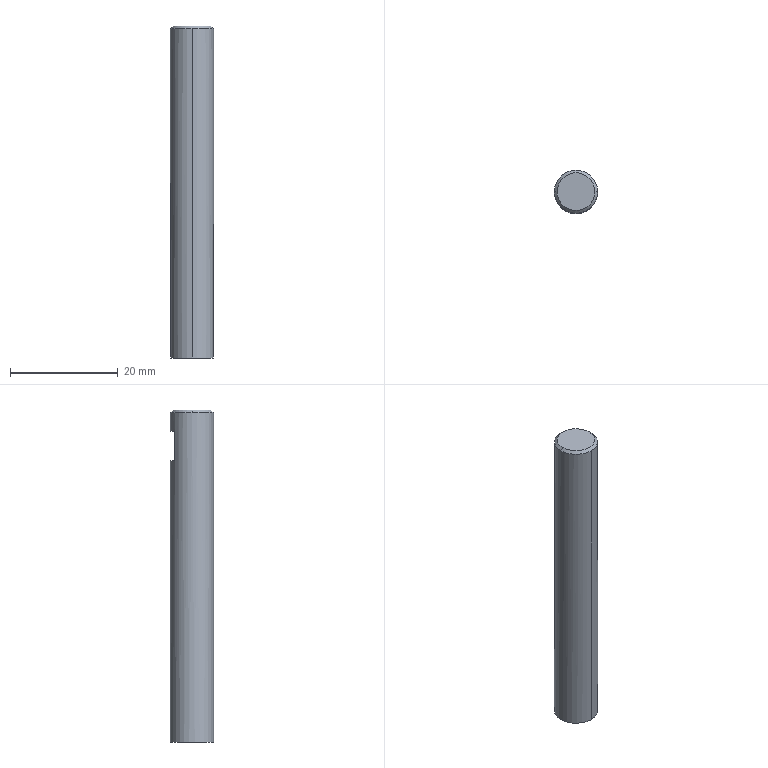Part | NX | 1 solid | 17 faces | box 8 x 8 x 61.5 mm | volume 2965 mm3 | cylinder 6 | cone 6 | plane 5 | commonest cylinder face diameters 3.3 x4 8 x2
STEP:
#1=CARTESIAN_POINT('',(-194.,196.7,-6.3));
#2=VERTEX_POINT('',#1);
#3=CARTESIAN_POINT('',(-190.,192.7,-6.3));
#4=VERTEX_POINT('',#3);
#5=CARTESIAN_POINT('',(-190.,196.7,-6.3));
#6=DIRECTION('',(0.,0.,1.));
#7=DIRECTION('',(1.,0.,0.));
#8=AXIS2_PLACEMENT_3D('',#5,#6,#7);
#9=CIRCLE('',#8,4.);
#10=EDGE_CURVE('',#2,#4,#9,.T.);
#11=ORIENTED_EDGE('',*,*,#10,.F.);
#12=CARTESIAN_POINT('',(-190.,200.7,-6.3));
#13=VERTEX_POINT('',#12);
#14=CARTESIAN_POINT('',(-190.,196.7,-6.3));
#15=DIRECTION('',(0.,0.,1.));
#16=DIRECTION('',(1.,0.,0.));
#17=AXIS2_PLACEMENT_3D('',#14,#15,#16);
#18=CIRCLE('',#17,4.);
#19=EDGE_CURVE('',#13,#2,#18,.T.);
#20=ORIENTED_EDGE('',*,*,#19,.F.);
#21=CARTESIAN_POINT('',(-190.,200.7,-9.7));
#22=VERTEX_POINT('',#21);
#23=CARTESIAN_POINT('',(-190.,200.7,-55.8));
#24=DIRECTION('',(0.,0.,1.));
#25=VECTOR('',#24,1000.);
#26=LINE('',#23,#25);
#27=EDGE_CURVE('',#13,#22,#26,.F.);
#28=ORIENTED_EDGE('',*,*,#27,.T.);
#29=CARTESIAN_POINT('',(-192.4,199.9,-9.7));
#30=VERTEX_POINT('',#29);
#31=CARTESIAN_POINT('',(-190.,196.7,-9.7));
#32=DIRECTION('',(0.,0.,1.));
#33=DIRECTION('',(0.,-1.,0.));
#34=AXIS2_PLACEMENT_3D('',#31,#32,#33);
#35=CIRCLE('',#34,4.);
#36=EDGE_CURVE('',#22,#30,#35,.T.);
#37=ORIENTED_EDGE('',*,*,#36,.T.);
#38=CARTESIAN_POINT('',(-192.4,199.9,-15.2));
#39=VERTEX_POINT('',#38);
#40=CARTESIAN_POINT('',(-192.4,199.9,-55.8));
#41=DIRECTION('',(0.,0.,1.));
#42=VECTOR('',#41,1000.);
#43=LINE('',#40,#42);
#44=EDGE_CURVE('',#39,#30,#43,.T.);
#45=ORIENTED_EDGE('',*,*,#44,.F.);
#46=CARTESIAN_POINT('',(-190.,200.7,-15.2));
#47=VERTEX_POINT('',#46);
#48=CARTESIAN_POINT('',(-190.,196.7,-15.2));
#49=DIRECTION('',(0.,0.,1.));
#50=DIRECTION('',(0.,-1.,0.));
#51=AXIS2_PLACEMENT_3D('',#48,#49,#50);
#52=CIRCLE('',#51,4.);
#53=EDGE_CURVE('',#47,#39,#52,.T.);
#54=ORIENTED_EDGE('',*,*,#53,.F.);
#55=CARTESIAN_POINT('',(-190.,200.7,-67.3));
#56=VERTEX_POINT('',#55);
#57=CARTESIAN_POINT('',(-190.,200.7,-55.8));
#58=DIRECTION('',(0.,0.,1.));
#59=VECTOR('',#58,1000.);
#60=LINE('',#57,#59);
#61=EDGE_CURVE('',#56,#47,#60,.T.);
#62=ORIENTED_EDGE('',*,*,#61,.F.);
#63=CARTESIAN_POINT('',(-190.,192.7,-67.3));
#64=VERTEX_POINT('',#63);
#65=CARTESIAN_POINT('',(-190.,196.7,-67.3));
#66=DIRECTION('',(0.,0.,1.));
#67=DIRECTION('',(0.,-1.,0.));
#68=AXIS2_PLACEMENT_3D('',#65,#66,#67);
#69=CIRCLE('',#68,4.);
#70=EDGE_CURVE('',#56,#64,#69,.T.);
#71=ORIENTED_EDGE('',*,*,#70,.T.);
#72=CARTESIAN_POINT('',(-190.,192.7,-55.8));
#73=DIRECTION('',(0.,0.,1.));
#74=VECTOR('',#73,1000.);
#75=LINE('',#72,#74);
#76=EDGE_CURVE('',#4,#64,#75,.F.);
#77=ORIENTED_EDGE('',*,*,#76,.F.);
#78=EDGE_LOOP('',(#11,#20,#28,#37,#45,#54,#62,#71,#77));
#79=FACE_BOUND('',#78,.T.);
#80=CARTESIAN_POINT('',(-190.,196.7,-55.8));
#81=DIRECTION('',(0.,0.,1.));
#82=DIRECTION('',(0.,-1.,0.));
#83=AXIS2_PLACEMENT_3D('',#80,#81,#82);
#84=CYLINDRICAL_SURFACE('',#83,4.);
#85=ADVANCED_FACE('',(#79),#84,.T.);
#86=ORIENTED_EDGE('',*,*,#70,.F.);
#87=CARTESIAN_POINT('',(-190.,196.7,-67.3));
#88=DIRECTION('',(0.,0.,1.));
#89=DIRECTION('',(0.,-1.,0.));
#90=AXIS2_PLACEMENT_3D('',#87,#88,#89);
#91=CIRCLE('',#90,4.);
#92=EDGE_CURVE('',#64,#56,#91,.T.);
#93=ORIENTED_EDGE('',*,*,#92,.F.);
#94=EDGE_LOOP('',(#86,#93));
#95=FACE_BOUND('',#94,.T.);
#96=CARTESIAN_POINT('',(-187.685,196.7,-67.3));
#97=VERTEX_POINT('',#96);
#98=CARTESIAN_POINT('',(-192.315,196.7,-67.3));
#99=VERTEX_POINT('',#98);
#100=CARTESIAN_POINT('',(-190.,196.7,-67.3));
#101=DIRECTION('',(0.,0.,-1.));
#102=DIRECTION('',(-1.,0.,0.));
#103=AXIS2_PLACEMENT_3D('',#100,#101,#102);
#104=CIRCLE('',#103,2.315);
#105=EDGE_CURVE('',#97,#99,#104,.T.);
#106=ORIENTED_EDGE('',*,*,#105,.F.);
#107=CARTESIAN_POINT('',(-190.,196.7,-67.3));
#108=DIRECTION('',(0.,0.,-1.));
#109=DIRECTION('',(-1.,0.,0.));
#110=AXIS2_PLACEMENT_3D('',#107,#108,#109);
#111=CIRCLE('',#110,2.315);
#112=EDGE_CURVE('',#99,#97,#111,.T.);
#113=ORIENTED_EDGE('',*,*,#112,.F.);
#114=EDGE_LOOP('',(#106,#113));
#115=FACE_BOUND('',#114,.T.);
#116=CARTESIAN_POINT('',(-181.498,197.784,-67.3));
#117=DIRECTION('',(0.,0.,-1.));
#118=DIRECTION('',(-1.,0.,0.));
#119=AXIS2_PLACEMENT_3D('',#116,#117,#118);
#120=PLANE('',#119);
#121=ADVANCED_FACE('',(#95,#115),#120,.T.);
#122=CARTESIAN_POINT('',(-186.5,196.7,-5.8));
#123=VERTEX_POINT('',#122);
#124=CARTESIAN_POINT('',(-193.5,196.7,-5.8));
#125=VERTEX_POINT('',#124);
#126=CARTESIAN_POINT('',(-190.,196.7,-5.8));
#127=DIRECTION('',(0.,0.,1.));
#128=DIRECTION('',(1.,0.,0.));
#129=AXIS2_PLACEMENT_3D('',#126,#127,#128);
#130=CIRCLE('',#129,3.5);
#131=EDGE_CURVE('',#123,#125,#130,.T.);
#132=ORIENTED_EDGE('',*,*,#131,.T.);
#133=CARTESIAN_POINT('',(-190.,196.7,-5.8));
#134=DIRECTION('',(0.,0.,1.));
#135=DIRECTION('',(1.,0.,0.));
#136=AXIS2_PLACEMENT_3D('',#133,#134,#135);
#137=CIRCLE('',#136,3.5);
#138=EDGE_CURVE('',#125,#123,#137,.T.);
#139=ORIENTED_EDGE('',*,*,#138,.T.);
#140=EDGE_LOOP('',(#132,#139));
#141=FACE_BOUND('',#140,.T.);
#142=CARTESIAN_POINT('',(-181.498,197.784,-5.8));
#143=DIRECTION('',(0.,0.,-1.));
#144=DIRECTION('',(-1.,0.,0.));
#145=AXIS2_PLACEMENT_3D('',#142,#143,#144);
#146=PLANE('',#145);
#147=ADVANCED_FACE('',(#141),#146,.F.);
#148=CARTESIAN_POINT('',(-187.6,199.9,-15.2));
#149=VERTEX_POINT('',#148);
#150=CARTESIAN_POINT('',(-187.6,199.9,-9.7));
#151=VERTEX_POINT('',#150);
#152=CARTESIAN_POINT('',(-187.6,199.9,-55.8));
#153=DIRECTION('',(0.,0.,1.));
#154=VECTOR('',#153,1000.);
#155=LINE('',#152,#154);
#156=EDGE_CURVE('',#149,#151,#155,.T.);
#157=ORIENTED_EDGE('',*,*,#156,.F.);
#158=CARTESIAN_POINT('',(-181.498,199.9,-15.2));
#159=DIRECTION('',(1.,0.,0.));
#160=VECTOR('',#159,1000.);
#161=LINE('',#158,#160);
#162=EDGE_CURVE('',#39,#149,#161,.T.);
#163=ORIENTED_EDGE('',*,*,#162,.F.);
#164=ORIENTED_EDGE('',*,*,#44,.T.);
#165=CARTESIAN_POINT('',(-181.498,199.9,-9.7));
#166=DIRECTION('',(1.,0.,0.));
#167=VECTOR('',#166,1000.);
#168=LINE('',#165,#167);
#169=EDGE_CURVE('',#30,#151,#168,.T.);
#170=ORIENTED_EDGE('',*,*,#169,.T.);
#171=EDGE_LOOP('',(#157,#163,#164,#170));
#172=FACE_BOUND('',#171,.T.);
#173=CARTESIAN_POINT('',(-192.646,199.9,-13.2));
#174=DIRECTION('',(0.,-1.,0.));
#175=DIRECTION('',(-1.,0.,0.));
#176=AXIS2_PLACEMENT_3D('',#173,#174,#175);
#177=PLANE('',#176);
#178=ADVANCED_FACE('',(#172),#177,.F.);
#179=ORIENTED_EDGE('',*,*,#10,.T.);
#180=CARTESIAN_POINT('',(-186.,196.7,-6.3));
#181=VERTEX_POINT('',#180);
#182=CARTESIAN_POINT('',(-190.,196.7,-6.3));
#183=DIRECTION('',(0.,0.,1.));
#184=DIRECTION('',(1.,0.,0.));
#185=AXIS2_PLACEMENT_3D('',#182,#183,#184);
#186=CIRCLE('',#185,4.);
#187=EDGE_CURVE('',#4,#181,#186,.T.);
#188=ORIENTED_EDGE('',*,*,#187,.T.);
#189=CARTESIAN_POINT('',(-186.5,196.7,-5.8));
#190=DIRECTION('',(0.7071,0.,-0.7071));
#191=VECTOR('',#190,1000.);
#192=LINE('',#189,#191);
#193=EDGE_CURVE('',#123,#181,#192,.T.);
#194=ORIENTED_EDGE('',*,*,#193,.F.);
#195=ORIENTED_EDGE('',*,*,#138,.F.);
#196=CARTESIAN_POINT('',(-193.5,196.7,-5.8));
#197=DIRECTION('',(-0.7071,0.,-0.7071));
#198=VECTOR('',#197,1000.);
#199=LINE('',#196,#198);
#200=EDGE_CURVE('',#125,#2,#199,.T.);
#201=ORIENTED_EDGE('',*,*,#200,.T.);
#202=EDGE_LOOP('',(#179,#188,#194,#195,#201));
#203=FACE_BOUND('',#202,.T.);
#204=CARTESIAN_POINT('',(-190.,196.7,-5.8));
#205=DIRECTION('',(0.,0.,-1.));
#206=DIRECTION('',(-1.,0.,0.));
#207=AXIS2_PLACEMENT_3D('',#204,#205,#206);
#208=CONICAL_SURFACE('',#207,3.5,0.7854);
#209=ADVANCED_FACE('',(#203),#208,.T.);
#210=ORIENTED_EDGE('',*,*,#162,.T.);
#211=CARTESIAN_POINT('',(-190.,196.7,-15.2));
#212=DIRECTION('',(0.,0.,1.));
#213=DIRECTION('',(0.,-1.,0.));
#214=AXIS2_PLACEMENT_3D('',#211,#212,#213);
#215=CIRCLE('',#214,4.);
#216=EDGE_CURVE('',#149,#47,#215,.T.);
#217=ORIENTED_EDGE('',*,*,#216,.T.);
#218=ORIENTED_EDGE('',*,*,#53,.T.);
#219=EDGE_LOOP('',(#210,#217,#218));
#220=FACE_BOUND('',#219,.T.);
#221=CARTESIAN_POINT('',(-185.645,200.992,-15.2));
#222=DIRECTION('',(0.,0.,1.));
#223=DIRECTION('',(1.,0.,0.));
#224=AXIS2_PLACEMENT_3D('',#221,#222,#223);
#225=PLANE('',#224);
#226=ADVANCED_FACE('',(#220),#225,.T.);
#227=ORIENTED_EDGE('',*,*,#36,.F.);
#228=CARTESIAN_POINT('',(-190.,196.7,-9.7));
#229=DIRECTION('',(0.,0.,1.));
#230=DIRECTION('',(0.,-1.,0.));
#231=AXIS2_PLACEMENT_3D('',#228,#229,#230);
#232=CIRCLE('',#231,4.);
#233=EDGE_CURVE('',#151,#22,#232,.T.);
#234=ORIENTED_EDGE('',*,*,#233,.F.);
#235=ORIENTED_EDGE('',*,*,#169,.F.);
#236=EDGE_LOOP('',(#227,#234,#235));
#237=FACE_BOUND('',#236,.T.);
#238=CARTESIAN_POINT('',(-185.645,200.992,-9.7));
#239=DIRECTION('',(0.,0.,1.));
#240=DIRECTION('',(1.,0.,0.));
#241=AXIS2_PLACEMENT_3D('',#238,#239,#240);
#242=PLANE('',#241);
#243=ADVANCED_FACE('',(#237),#242,.F.);
#244=CARTESIAN_POINT('',(-188.35,196.7,-66.916));
#245=VERTEX_POINT('',#244);
#246=CARTESIAN_POINT('',(-191.65,196.7,-66.916));
#247=VERTEX_POINT('',#246);
#248=CARTESIAN_POINT('',(-190.,196.7,-66.916));
#249=DIRECTION('',(0.,0.,-1.));
#250=DIRECTION('',(-1.,0.,0.));
#251=AXIS2_PLACEMENT_3D('',#248,#249,#250);
#252=CIRCLE('',#251,1.65);
#253=EDGE_CURVE('',#245,#247,#252,.T.);
#254=ORIENTED_EDGE('',*,*,#253,.T.);
#255=CARTESIAN_POINT('',(-191.65,196.7,-59.3));
#256=VERTEX_POINT('',#255);
#257=CARTESIAN_POINT('',(-191.65,196.7,-67.3));
#258=DIRECTION('',(0.,0.,-1.));
#259=VECTOR('',#258,1000.);
#260=LINE('',#257,#259);
#261=EDGE_CURVE('',#247,#256,#260,.F.);
#262=ORIENTED_EDGE('',*,*,#261,.T.);
#263=CARTESIAN_POINT('',(-188.35,196.7,-59.3));
#264=VERTEX_POINT('',#263);
#265=CARTESIAN_POINT('',(-190.,196.7,-59.3));
#266=DIRECTION('',(0.,0.,-1.));
#267=DIRECTION('',(-1.,0.,0.));
#268=AXIS2_PLACEMENT_3D('',#265,#266,#267);
#269=CIRCLE('',#268,1.65);
#270=EDGE_CURVE('',#264,#256,#269,.T.);
#271=ORIENTED_EDGE('',*,*,#270,.F.);
#272=CARTESIAN_POINT('',(-188.35,196.7,-67.3));
#273=DIRECTION('',(0.,0.,-1.));
#274=VECTOR('',#273,1000.);
#275=LINE('',#272,#274);
#276=EDGE_CURVE('',#245,#264,#275,.F.);
#277=ORIENTED_EDGE('',*,*,#276,.F.);
#278=EDGE_LOOP('',(#254,#262,#271,#277));
#279=FACE_BOUND('',#278,.T.);
#280=CARTESIAN_POINT('',(-190.,196.7,-67.3));
#281=DIRECTION('',(0.,0.,-1.));
#282=DIRECTION('',(-1.,0.,0.));
#283=AXIS2_PLACEMENT_3D('',#280,#281,#282);
#284=CYLINDRICAL_SURFACE('',#283,1.65);
#285=ADVANCED_FACE('',(#279),#284,.F.);
#286=ORIENTED_EDGE('',*,*,#270,.T.);
#287=CARTESIAN_POINT('',(-191.65,196.7,-55.1));
#288=VERTEX_POINT('',#287);
#289=CARTESIAN_POINT('',(-191.65,196.7,-67.3));
#290=DIRECTION('',(0.,0.,-1.));
#291=VECTOR('',#290,1000.);
#292=LINE('',#289,#291);
#293=EDGE_CURVE('',#256,#288,#292,.F.);
#294=ORIENTED_EDGE('',*,*,#293,.T.);
#295=CARTESIAN_POINT('',(-188.35,196.7,-55.1));
#296=VERTEX_POINT('',#295);
#297=CARTESIAN_POINT('',(-190.,196.7,-55.1));
#298=DIRECTION('',(0.,0.,-1.));
#299=DIRECTION('',(-1.,0.,0.));
#300=AXIS2_PLACEMENT_3D('',#297,#298,#299);
#301=CIRCLE('',#300,1.65);
#302=EDGE_CURVE('',#296,#288,#301,.T.);
#303=ORIENTED_EDGE('',*,*,#302,.F.);
#304=CARTESIAN_POINT('',(-188.35,196.7,-67.3));
#305=DIRECTION('',(0.,0.,-1.));
#306=VECTOR('',#305,1000.);
#307=LINE('',#304,#306);
#308=EDGE_CURVE('',#264,#296,#307,.F.);
#309=ORIENTED_EDGE('',*,*,#308,.F.);
#310=EDGE_LOOP('',(#286,#294,#303,#309));
#311=FACE_BOUND('',#310,.T.);
#312=CARTESIAN_POINT('',(-190.,196.7,-67.3));
#313=DIRECTION('',(0.,0.,-1.));
#314=DIRECTION('',(-1.,0.,0.));
#315=AXIS2_PLACEMENT_3D('',#312,#313,#314);
#316=CYLINDRICAL_SURFACE('',#315,1.65);
#317=ADVANCED_FACE('',(#311),#316,.F.);
#318=ORIENTED_EDGE('',*,*,#302,.T.);
#319=CARTESIAN_POINT('',(-190.,196.7,-54.109));
#320=VERTEX_POINT('',#319);
#321=CARTESIAN_POINT('',(-191.65,196.7,-55.1));
#322=DIRECTION('',(-0.8572,0.,-0.515));
#323=VECTOR('',#322,1000.);
#324=LINE('',#321,#323);
#325=EDGE_CURVE('',#320,#288,#324,.T.);
#326=ORIENTED_EDGE('',*,*,#325,.F.);
#327=CARTESIAN_POINT('',(-188.35,196.7,-55.1));
#328=DIRECTION('',(0.8572,0.,-0.515));
#329=VECTOR('',#328,1000.);
#330=LINE('',#327,#329);
#331=EDGE_CURVE('',#320,#296,#330,.T.);
#332=ORIENTED_EDGE('',*,*,#331,.T.);
#333=EDGE_LOOP('',(#318,#326,#332));
#334=FACE_BOUND('',#333,.T.);
#335=CARTESIAN_POINT('',(-190.,196.7,-55.1));
#336=DIRECTION('',(0.,0.,-1.));
#337=DIRECTION('',(-1.,0.,0.));
#338=AXIS2_PLACEMENT_3D('',#335,#336,#337);
#339=CONICAL_SURFACE('',#338,1.65,1.03);
#340=ADVANCED_FACE('',(#334),#339,.F.);
#341=ORIENTED_EDGE('',*,*,#253,.F.);
#342=CARTESIAN_POINT('',(-188.35,196.7,-66.916));
#343=DIRECTION('',(0.866,0.,-0.5));
#344=VECTOR('',#343,1000.);
#345=LINE('',#342,#344);
#346=EDGE_CURVE('',#97,#245,#345,.F.);
#347=ORIENTED_EDGE('',*,*,#346,.F.);
#348=ORIENTED_EDGE('',*,*,#105,.T.);
#349=CARTESIAN_POINT('',(-191.65,196.7,-66.916));
#350=DIRECTION('',(-0.866,0.,-0.5));
#351=VECTOR('',#350,1000.);
#352=LINE('',#349,#351);
#353=EDGE_CURVE('',#99,#247,#352,.F.);
#354=ORIENTED_EDGE('',*,*,#353,.T.);
#355=EDGE_LOOP('',(#341,#347,#348,#354));
#356=FACE_BOUND('',#355,.T.);
#357=CARTESIAN_POINT('',(-190.,196.7,-66.916));
#358=DIRECTION('',(0.,0.,-1.));
#359=DIRECTION('',(-1.,0.,0.));
#360=AXIS2_PLACEMENT_3D('',#357,#358,#359);
#361=CONICAL_SURFACE('',#360,1.65,1.047);
#362=ADVANCED_FACE('',(#356),#361,.F.);
#363=ORIENTED_EDGE('',*,*,#331,.F.);
#364=ORIENTED_EDGE('',*,*,#325,.T.);
#365=CARTESIAN_POINT('',(-190.,196.7,-55.1));
#366=DIRECTION('',(0.,0.,-1.));
#367=DIRECTION('',(-1.,0.,0.));
#368=AXIS2_PLACEMENT_3D('',#365,#366,#367);
#369=CIRCLE('',#368,1.65);
#370=EDGE_CURVE('',#288,#296,#369,.T.);
#371=ORIENTED_EDGE('',*,*,#370,.T.);
#372=EDGE_LOOP('',(#363,#364,#371));
#373=FACE_BOUND('',#372,.T.);
#374=CARTESIAN_POINT('',(-190.,196.7,-55.1));
#375=DIRECTION('',(0.,0.,-1.));
#376=DIRECTION('',(-1.,0.,0.));
#377=AXIS2_PLACEMENT_3D('',#374,#375,#376);
#378=CONICAL_SURFACE('',#377,1.65,1.03);
#379=ADVANCED_FACE('',(#373),#378,.F.);
#380=ORIENTED_EDGE('',*,*,#293,.F.);
#381=CARTESIAN_POINT('',(-190.,196.7,-59.3));
#382=DIRECTION('',(0.,0.,-1.));
#383=DIRECTION('',(-1.,0.,0.));
#384=AXIS2_PLACEMENT_3D('',#381,#382,#383);
#385=CIRCLE('',#384,1.65);
#386=EDGE_CURVE('',#256,#264,#385,.T.);
#387=ORIENTED_EDGE('',*,*,#386,.T.);
#388=ORIENTED_EDGE('',*,*,#308,.T.);
#389=ORIENTED_EDGE('',*,*,#370,.F.);
#390=EDGE_LOOP('',(#380,#387,#388,#389));
#391=FACE_BOUND('',#390,.T.);
#392=CARTESIAN_POINT('',(-190.,196.7,-67.3));
#393=DIRECTION('',(0.,0.,-1.));
#394=DIRECTION('',(-1.,0.,0.));
#395=AXIS2_PLACEMENT_3D('',#392,#393,#394);
#396=CYLINDRICAL_SURFACE('',#395,1.65);
#397=ADVANCED_FACE('',(#391),#396,.F.);
#398=ORIENTED_EDGE('',*,*,#261,.F.);
#399=CARTESIAN_POINT('',(-190.,196.7,-66.916));
#400=DIRECTION('',(0.,0.,-1.));
#401=DIRECTION('',(-1.,0.,0.));
#402=AXIS2_PLACEMENT_3D('',#399,#400,#401);
#403=CIRCLE('',#402,1.65);
#404=EDGE_CURVE('',#247,#245,#403,.T.);
#405=ORIENTED_EDGE('',*,*,#404,.T.);
#406=ORIENTED_EDGE('',*,*,#276,.T.);
#407=ORIENTED_EDGE('',*,*,#386,.F.);
#408=EDGE_LOOP('',(#398,#405,#406,#407));
#409=FACE_BOUND('',#408,.T.);
#410=CARTESIAN_POINT('',(-190.,196.7,-67.3));
#411=DIRECTION('',(0.,0.,-1.));
#412=DIRECTION('',(-1.,0.,0.));
#413=AXIS2_PLACEMENT_3D('',#410,#411,#412);
#414=CYLINDRICAL_SURFACE('',#413,1.65);
#415=ADVANCED_FACE('',(#409),#414,.F.);
#416=ORIENTED_EDGE('',*,*,#353,.F.);
#417=ORIENTED_EDGE('',*,*,#112,.T.);
#418=ORIENTED_EDGE('',*,*,#346,.T.);
#419=ORIENTED_EDGE('',*,*,#404,.F.);
#420=EDGE_LOOP('',(#416,#417,#418,#419));
#421=FACE_BOUND('',#420,.T.);
#422=CARTESIAN_POINT('',(-190.,196.7,-66.916));
#423=DIRECTION('',(0.,0.,-1.));
#424=DIRECTION('',(-1.,0.,0.));
#425=AXIS2_PLACEMENT_3D('',#422,#423,#424);
#426=CONICAL_SURFACE('',#425,1.65,1.047);
#427=ADVANCED_FACE('',(#421),#426,.F.);
#428=ORIENTED_EDGE('',*,*,#131,.F.);
#429=ORIENTED_EDGE('',*,*,#193,.T.);
#430=CARTESIAN_POINT('',(-190.,196.7,-6.3));
#431=DIRECTION('',(0.,0.,1.));
#432=DIRECTION('',(1.,0.,0.));
#433=AXIS2_PLACEMENT_3D('',#430,#431,#432);
#434=CIRCLE('',#433,4.);
#435=EDGE_CURVE('',#181,#13,#434,.T.);
#436=ORIENTED_EDGE('',*,*,#435,.T.);
#437=ORIENTED_EDGE('',*,*,#19,.T.);
#438=ORIENTED_EDGE('',*,*,#200,.F.);
#439=EDGE_LOOP('',(#428,#429,#436,#437,#438));
#440=FACE_BOUND('',#439,.T.);
#441=CARTESIAN_POINT('',(-190.,196.7,-5.8));
#442=DIRECTION('',(0.,0.,-1.));
#443=DIRECTION('',(-1.,0.,0.));
#444=AXIS2_PLACEMENT_3D('',#441,#442,#443);
#445=CONICAL_SURFACE('',#444,3.5,0.7854);
#446=ADVANCED_FACE('',(#440),#445,.T.);
#447=ORIENTED_EDGE('',*,*,#76,.T.);
#448=ORIENTED_EDGE('',*,*,#92,.T.);
#449=ORIENTED_EDGE('',*,*,#61,.T.);
#450=ORIENTED_EDGE('',*,*,#216,.F.);
#451=ORIENTED_EDGE('',*,*,#156,.T.);
#452=ORIENTED_EDGE('',*,*,#233,.T.);
#453=ORIENTED_EDGE('',*,*,#27,.F.);
#454=ORIENTED_EDGE('',*,*,#435,.F.);
#455=ORIENTED_EDGE('',*,*,#187,.F.);
#456=EDGE_LOOP('',(#447,#448,#449,#450,#451,#452,#453,#454,#455));
#457=FACE_BOUND('',#456,.T.);
#458=CARTESIAN_POINT('',(-190.,196.7,-55.8));
#459=DIRECTION('',(0.,0.,1.));
#460=DIRECTION('',(0.,-1.,0.));
#461=AXIS2_PLACEMENT_3D('',#458,#459,#460);
#462=CYLINDRICAL_SURFACE('',#461,4.);
#463=ADVANCED_FACE('',(#457),#462,.T.);
#464=CLOSED_SHELL('',(#85,#121,#147,#178,#209,#226,#243,#285,#317,#340,#362,#379,#397,#415,#427,#446,#463));
#465=MANIFOLD_SOLID_BREP('',#464);
#466=(LENGTH_UNIT()NAMED_UNIT(*)SI_UNIT(.MILLI.,.METRE.));
#467=UNCERTAINTY_MEASURE_WITH_UNIT(LENGTH_MEASURE(0.00001),#466,'','');
#468=(NAMED_UNIT(*)PLANE_ANGLE_UNIT()SI_UNIT($,.RADIAN.));
#469=(NAMED_UNIT(*)SI_UNIT($,.STERADIAN.)SOLID_ANGLE_UNIT());
#470=(GEOMETRIC_REPRESENTATION_CONTEXT(3)GLOBAL_UNCERTAINTY_ASSIGNED_CONTEXT((#467))GLOBAL_UNIT_ASSIGNED_CONTEXT((#466,#468,#469))REPRESENTATION_CONTEXT('',''));
#471=ADVANCED_BREP_SHAPE_REPRESENTATION('',(#465),#470);